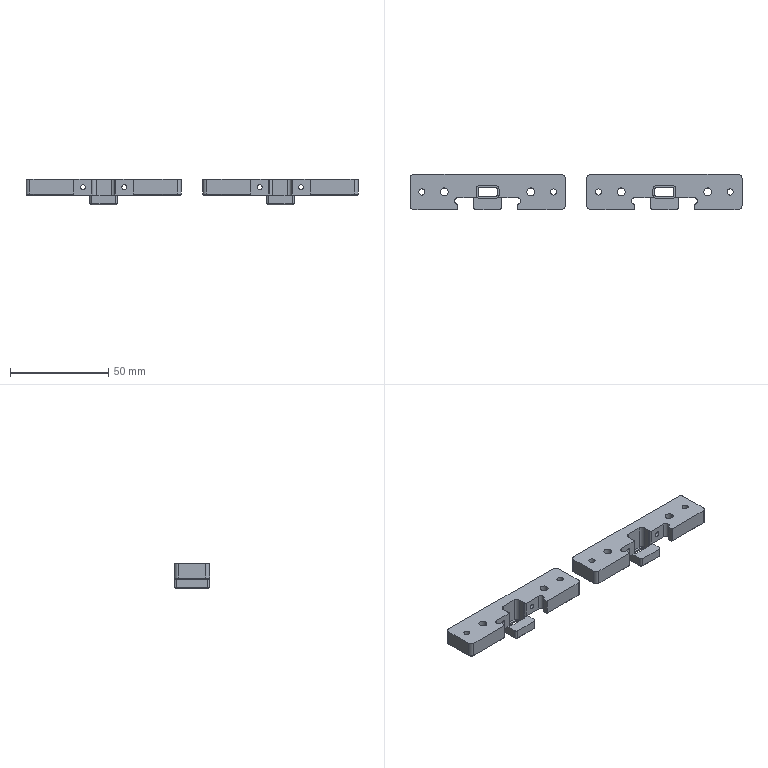NC program | NX | posted with a generic post | part box 169 x 18 x 12.9 mm
Whole program:
N10 G17 G21 G94 G90
(FLOOR_WALL_COPY , TOOL : D63)
N12 T01 M6
N14 G54
N16 G17 G0 G90 X-121. Y0. S6500 M3
N18 G43 Z30. H1
N20 Z4.
N22 G94 G1 Z1. F1250.
N24 X-118.
N26 X118.
N28 X121.
N30 Z4.
N32 G0 Z30.
N34 X-121.
N36 Z3.
N38 G1 Z0.
N40 X-118.
N42 X118.
N44 X121.
N46 Z3.
N48 G0 Z30.
N50 M5
(CAVITY_MILL_COPY_COPY_COPY_1 , TOOL : D6)
N52 T06 M6
N54 G54
N56 G17 G0 G90 X-2.829 Y15.196 S9500 M3
N58 G43 Z30. H6
N60 Z-0.6
N62 G94 G1 X-0.866 Y11.796 F1000.
N64 G3 X0. Y11.296 R1.
N66 G1 X35.32 F2000.
N68 G2 X39. Y12.94 R4.94
N70 G1 X51.
N72 G2 X54.68 Y11.296 R4.94
N74 G1 X86.504
N76 G2 X86.796 Y11.004 R0.292
N78 G1 Y-11.004
N80 G2 X86.504 Y-11.296 R0.292
N82 G1 X55.94
N84 Y-7.096
N86 Y7.096
N88 X82.596
N90 Y-7.096
N92 X55.94
N94 X60.14 Y-2.896
N96 Y2.896
N98 X78.396
N100 Y-2.896
N102 X60.14
N104 X62.84 Y-0.196
N106 Y0.196
N108 X75.696
N110 Y-0.196
N112 X62.84
N114 X55.94 Y-7.096
N116 Y-11.296
N118 X54.68
N120 G2 X51. Y-12.94 R4.94
N122 G1 X39.
N124 G2 X35.32 Y-11.296 R4.94
N126 G1 X-35.32
N128 G2 X-39. Y-12.94 R4.94
N130 G1 X-51.
N132 G2 X-54.68 Y-11.296 R4.94
N134 G1 X-86.504
N136 G2 X-86.796 Y-11.004 R0.292
N138 G1 Y11.004
N140 G2 X-86.504 Y11.296 R0.292
N142 G1 X-55.94
N144 Y7.096
N146 Y-7.096
N148 X-82.596
N150 Y7.096
N152 X-55.94
N154 X-60.14 Y2.896
N156 Y-2.896
N158 X-78.396
N160 Y2.896
N162 X-60.14
N164 X-62.84 Y0.196
N166 Y-0.196
N168 X-75.696
N170 Y0.196
N172 X-62.84
N174 X-55.94 Y7.096
N176 Y11.296
N178 X-54.68
N180 G2 X-51. Y12.94 R4.94
N182 G1 X-39.
N184 G2 X-35.32 Y11.296 R4.94
N186 G1 X0.
N188 Y7.096
N190 X34.06
N192 Y-7.096
N194 X34.9
N196 Y8.
N198 G2 X39. Y12.1 R4.1
N200 G1 X51.
N202 G2 X55.1 Y8. R4.1
N204 G1 Y-8.
N206 G2 X51. Y-12.1 R4.1
N208 G1 X39.
N210 G2 X34.9 Y-8. R4.1
N212 G1 Y-7.096
N214 X34.06
N216 X-34.06
N218 Y7.096
N220 X-34.9
N222 Y-8.
N224 G2 X-39. Y-12.1 R4.1
N226 G1 X-51.
N228 G2 X-55.1 Y-8. R4.1
N230 G1 Y8.
N232 G2 X-51. Y12.1 R4.1
N234 G1 X-39.
N236 G2 X-34.9 Y8. R4.1
N238 G1 Y7.096
N240 X-34.06
N242 X0.
N244 Y2.896
N246 X29.86
N248 Y-2.896
N250 X-29.86
N252 Y2.896
N254 X0.
N256 Y0.196
N258 X27.16
N260 Y-0.196
N262 X-27.16
N264 Y0.196
N266 X0.
N268 G3 X0.866 Y0.696 R1.
N270 G0 Z30.
N272 X-2.829 Y15.196
N274 Z-1.2
N276 G1 X-0.866 Y11.796 F1000.
N278 G3 X0. Y11.296 R1.
N280 G1 X35.32 F2000.
N282 G2 X39. Y12.94 R4.94
N284 G1 X51.
N286 G2 X54.68 Y11.296 R4.94
N288 G1 X86.504
N290 G2 X86.796 Y11.003 R0.292
N292 G1 Y-11.003
N294 G2 X86.504 Y-11.296 R0.292
N296 G1 X55.94
N298 Y-7.096
N300 Y7.096
N302 X82.596
N304 Y-7.096
N306 X55.94
N308 X60.14 Y-2.896
N310 Y2.896
N312 X78.396
N314 Y-2.896
N316 X60.14
N318 X62.84 Y-0.196
N320 Y0.196
N322 X75.696
N324 Y-0.196
N326 X62.84
N328 X55.94 Y-7.096
N330 Y-11.296
N332 X54.68
N334 G2 X51. Y-12.94 R4.94
N336 G1 X39.
N338 G2 X35.32 Y-11.296 R4.94
N340 G1 X-35.32
N342 G2 X-39. Y-12.94 R4.94
N344 G1 X-51.
N346 G2 X-54.68 Y-11.296 R4.94
N348 G1 X-86.504
N350 G2 X-86.796 Y-11.003 R0.292
N352 G1 Y11.003
N354 G2 X-86.504 Y11.296 R0.292
N356 G1 X-55.94
N358 Y7.096
N360 Y-7.096
N362 X-82.596
N364 Y7.096
N366 X-55.94
N368 X-60.14 Y2.896
N370 Y-2.896
N372 X-78.396
N374 Y2.896
N376 X-60.14
N378 X-62.84 Y0.196
N380 Y-0.196
N382 X-75.696
N384 Y0.196
N386 X-62.84
N388 X-55.94 Y7.096
N390 Y11.296
N392 X-54.68
N394 G2 X-51. Y12.94 R4.94
N396 G1 X-39.
N398 G2 X-35.32 Y11.296 R4.94
N400 G1 X0.
N402 Y7.096
N404 X34.06
N406 Y-7.096
N408 X34.9
N410 Y8.
N412 G2 X39. Y12.1 R4.1
N414 G1 X51.
N416 G2 X55.1 Y8. R4.1
N418 G1 Y-8.
N420 G2 X51. Y-12.1 R4.1
N422 G1 X39.
N424 G2 X34.9 Y-8. R4.1
N426 G1 Y-7.096
N428 X34.06
N430 X-34.06
N432 Y7.096
N434 X-34.9
N436 Y-8.
N438 G2 X-39. Y-12.1 R4.1
N440 G1 X-51.
N442 G2 X-55.1 Y-8. R4.1
N444 G1 Y8.
N446 G2 X-51. Y12.1 R4.1
N448 G1 X-39.
N450 G2 X-34.9 Y8. R4.1
N452 G1 Y7.096
N454 X-34.06
N456 X0.
N458 Y2.896
N460 X29.86
N462 Y-2.896
N464 X-29.86
N466 Y2.896
N468 X0.
N470 Y0.196
N472 X27.16
N474 Y-0.196
N476 X-27.16
N478 Y0.196
N480 X0.
N482 G3 X0.866 Y0.696 R1.
N484 G0 Z30.
N486 X-2.829 Y15.196
N488 Z-1.8
N490 G1 X-0.866 Y11.796 F1000.
N492 G3 X0. Y11.296 R1.
N494 G1 X35.32 F2000.
N496 G2 X39. Y12.94 R4.94
N498 G1 X51.
N500 G2 X54.68 Y11.296 R4.94
N502 G1 X86.504
N504 G2 X86.796 Y11.003 R0.293
N506 G1 Y-11.003
N508 G2 X86.504 Y-11.296 R0.293
N510 G1 X55.94
N512 Y-7.096
N514 Y7.096
N516 X82.596
N518 Y-7.096
N520 X55.94
N522 X60.14 Y-2.896
N524 Y2.896
N526 X78.396
N528 Y-2.896
N530 X60.14
N532 X62.84 Y-0.196
N534 Y0.196
N536 X75.696
N538 Y-0.196
N540 X62.84
N542 X55.94 Y-7.096
N544 Y-11.296
N546 X54.68
N548 G2 X51. Y-12.94 R4.94
N550 G1 X39.
N552 G2 X35.32 Y-11.296 R4.94
N554 G1 X-35.32
N556 G2 X-39. Y-12.94 R4.94
N558 G1 X-51.
N560 G2 X-54.68 Y-11.296 R4.94
N562 G1 X-86.504
N564 G2 X-86.796 Y-11.003 R0.293
N566 G1 Y11.003
N568 G2 X-86.504 Y11.296 R0.293
N570 G1 X-55.94
N572 Y7.096
N574 Y-7.096
N576 X-82.596
N578 Y7.096
N580 X-55.94
N582 X-60.14 Y2.896
N584 Y-2.896
N586 X-78.396
N588 Y2.896
N590 X-60.14
N592 X-62.84 Y0.196
N594 Y-0.196
N596 X-75.696
N598 Y0.196
N600 X-62.84
N602 X-55.94 Y7.096
N604 Y11.296
N606 X-54.68
N608 G2 X-51. Y12.94 R4.94
N610 G1 X-39.
N612 G2 X-35.32 Y11.296 R4.94
N614 G1 X0.
N616 Y7.096
N618 X34.06
N620 Y-7.096
N622 X34.9
N624 Y8.
N626 G2 X39. Y12.1 R4.1
N628 G1 X51.
N630 G2 X55.1 Y8. R4.1
N632 G1 Y-8.
N634 G2 X51. Y-12.1 R4.1
N636 G1 X39.
N638 G2 X34.9 Y-8. R4.1
N640 G1 Y-7.096
N642 X34.06
N644 X-34.06
N646 Y7.096
N648 X-34.9
N650 Y-8.
N652 G2 X-39. Y-12.1 R4.1
N654 G1 X-51.
N656 G2 X-55.1 Y-8. R4.1
N658 G1 Y8.
N660 G2 X-51. Y12.1 R4.1
N662 G1 X-39.
N664 G2 X-34.9 Y8. R4.1
N666 G1 Y7.096
N668 X-34.06
N670 X0.
N672 Y2.896
N674 X29.86
N676 Y-2.896
N678 X-29.86
N680 Y2.896
N682 X0.
N684 Y0.196
N686 X27.16
N688 Y-0.196
N690 X-27.16
N692 Y0.196
N694 X0.
N696 G3 X0.866 Y0.696 R1.
N698 G0 Z30.
N700 X-2.829 Y15.196
N702 Z-2.4
N704 G1 X-0.866 Y11.796 F1000.
N706 G3 X0. Y11.296 R1.
N708 G1 X35.321 F2000.
N710 G2 X39. Y12.94 R4.94
N712 G1 X51.
N714 G2 X54.679 Y11.296 R4.94
N716 G1 X86.503
N718 G2 X86.797 Y11.003 R0.293
N720 G1 Y-11.003
N722 G2 X86.503 Y-11.296 R0.293
N724 G1 X55.94
N726 Y-7.096
N728 Y7.096
N730 X82.597
N732 Y-7.096
N734 X55.94
N736 X60.14 Y-2.896
N738 Y2.896
N740 X78.397
N742 Y-2.896
N744 X60.14
N746 X62.84 Y-0.196
N748 Y0.196
N750 X75.697
N752 Y-0.196
N754 X62.84
N756 X60.14 Y-2.896
N758 X55.94 Y-7.096
N760 Y-11.296
N762 X54.679
N764 G2 X51. Y-12.94 R4.94
N766 G1 X39.
N768 G2 X35.321 Y-11.296 R4.94
N770 G1 X-35.321
N772 G2 X-39. Y-12.94 R4.94
N774 G1 X-51.
N776 G2 X-54.679 Y-11.296 R4.94
N778 G1 X-86.504
N780 G2 X-86.797 Y-11.003 R0.293
N782 G1 Y11.003
N784 G2 X-86.504 Y11.296 R0.293
N786 G1 X-55.94
N788 Y7.096
N790 Y-7.096
N792 X-82.597
N794 Y7.096
N796 X-55.94
N798 X-60.14 Y2.896
N800 Y-2.896
N802 X-78.397
N804 Y2.896
N806 X-60.14
N808 X-62.84 Y0.196
N810 Y-0.196
N812 X-75.697
N814 Y0.196
N816 X-62.84
N818 X-55.94 Y7.096
N820 Y11.296
N822 X-54.679
N824 G2 X-51. Y12.94 R4.94
N826 G1 X-39.
N828 G2 X-35.321 Y11.296 R4.94
N830 G1 X0.
N832 Y7.096
N834 X34.06
N836 Y-7.096
N838 X34.9
N840 Y8.
N842 G2 X39. Y12.1 R4.1
N844 G1 X51.
N846 G2 X55.1 Y8. R4.1
N848 G1 Y-8.
N850 G2 X51. Y-12.1 R4.1
N852 G1 X39.
N854 G2 X34.9 Y-8. R4.1
N856 G1 Y-7.096
N858 X34.06
N860 X-34.06
N862 Y7.096
N864 X-34.9
N866 Y-8.
N868 G2 X-39. Y-12.1 R4.1
N870 G1 X-51.
N872 G2 X-55.1 Y-8. R4.1
N874 G1 Y8.
N876 G2 X-51. Y12.1 R4.1
N878 G1 X-39.
N880 G2 X-34.9 Y8. R4.1
N882 G1 Y7.096
N884 X-34.06
N886 X0.
N888 Y2.896
N890 X29.86
N892 Y-2.896
N894 X-29.86
N896 Y2.896
N898 X0.
N900 Y0.196
N902 X27.16
N904 Y-0.196
N906 X-27.16
N908 Y0.196
N910 X0.
N912 G3 X0.866 Y0.696 R1.
N914 G0 Z30.
N916 X-2.829 Y15.196
N918 Z-3.
N920 G1 X-0.866 Y11.796 F1000.
N922 G3 X0. Y11.296 R1.
N924 G1 X35.321 F2000.
N926 G2 X39. Y12.94 R4.94
N928 G1 X51.
N930 G2 X54.679 Y11.296 R4.94
N932 G1 X86.503
N934 G2 X86.797 Y11.003 R0.293
N936 G1 Y-11.003
N938 G2 X86.503 Y-11.296 R0.293
N940 G1 X55.94
N942 Y-7.096
N944 Y7.096
N946 X82.597
N948 Y-7.096
N950 X55.94
N952 X60.14 Y-2.896
N954 Y2.896
N956 X78.397
N958 Y-2.896
N960 X60.14
N962 X62.84 Y-0.196
N964 Y0.196
N966 X75.697
N968 Y-0.196
N970 X62.84
N972 X55.94 Y-7.096
N974 Y-11.296
N976 X54.679
N978 G2 X51. Y-12.94 R4.94
N980 G1 X39.
N982 G2 X35.321 Y-11.296 R4.94
N984 G1 X-35.321
N986 G2 X-39. Y-12.94 R4.94
N988 G1 X-51.
N990 G2 X-54.679 Y-11.296 R4.94
N992 G1 X-86.503
N994 G2 X-86.797 Y-11.003 R0.293
N996 G1 Y11.003
N998 G2 X-86.503 Y11.296 R0.293
N1000 G1 X-55.94
N1002 Y7.096
N1004 Y-7.096
N1006 X-82.597
N1008 Y7.096
N1010 X-55.94
N1012 X-60.14 Y2.896
N1014 Y-2.896
N1016 X-78.397
N1018 Y2.896
N1020 X-60.14
N1022 X-62.84 Y0.196
N1024 Y-0.196
N1026 X-75.697
N1028 Y0.196
N1030 X-62.84
N1032 X-55.94 Y7.096
N1034 Y11.296
N1036 X-54.679
N1038 G2 X-51. Y12.94 R4.94
N1040 G1 X-39.
N1042 G2 X-35.321 Y11.296 R4.94
N1044 G1 X0.
N1046 Y7.096
N1048 X34.06
N1050 Y-7.096
N1052 X34.9
N1054 Y8.
N1056 G2 X39. Y12.1 R4.1
N1058 G1 X51.
N1060 G2 X55.1 Y8. R4.1
N1062 G1 Y-8.
N1064 G2 X51. Y-12.1 R4.1
N1066 G1 X39.
N1068 G2 X34.9 Y-8. R4.1
N1070 G1 Y-7.096
N1072 X34.06
N1074 X-34.06
N1076 Y7.096
N1078 X-34.9
N1080 Y-8.
N1082 G2 X-39. Y-12.1 R4.1
N1084 G1 X-51.
N1086 G2 X-55.1 Y-8. R4.1
N1088 G1 Y8.
N1090 G2 X-51. Y12.1 R4.1
N1092 G1 X-39.
N1094 G2 X-34.9 Y8. R4.1
N1096 G1 Y7.096
N1098 X-34.06
N1100 X0.
N1102 Y2.896
N1104 X29.86
N1106 Y-2.896
N1108 X-29.86
N1110 Y2.896
N1112 X0.
N1114 Y0.196
N1116 X27.16
N1118 Y-0.196
N1120 X-27.16
N1122 Y0.196
N1124 X0.
N1126 G3 X0.866 Y0.696 R1.
N1128 G0 Z30.
N1130 X-2.829 Y15.197
N1132 Z-3.6
N1134 G1 X-0.866 Y11.797 F1000.
N1136 G3 X0. Y11.297 R1.
N1138 G1 X35.321 F2000.
N1140 G2 X39. Y12.94 R4.94
N1142 G1 X51.
N1144 G2 X54.679 Y11.297 R4.94
N1146 G1 X86.503
N1148 G2 X86.797 Y11.003 R0.294
N1150 G1 Y-11.003
N1152 G2 X86.503 Y-11.297 R0.294
N1154 G1 X55.94
N1156 Y-7.097
N1158 Y7.097
N1160 X82.597
N1162 Y-7.097
N1164 X55.94
N1166 X60.14 Y-2.897
N1168 Y2.897
N1170 X78.397
N1172 Y-2.897
N1174 X60.14
N1176 X62.84 Y-0.197
N1178 Y0.197
N1180 X75.697
N1182 Y-0.197
N1184 X62.84
N1186 X55.94 Y-7.097
N1188 Y-11.297
N1190 X54.679
N1192 G2 X51. Y-12.94 R4.94
N1194 G1 X39.
N1196 G2 X35.321 Y-11.297 R4.94
N1198 G1 X-35.321
N1200 G2 X-39. Y-12.94 R4.94
N1202 G1 X-51.
N1204 G2 X-54.679 Y-11.297 R4.94
N1206 G1 X-86.503
N1208 G2 X-86.797 Y-11.003 R0.294
N1210 G1 Y11.003
N1212 G2 X-86.503 Y11.297 R0.294
N1214 G1 X-55.94
N1216 Y7.097
N1218 Y-7.097
N1220 X-82.597
N1222 Y7.097
N1224 X-55.94
N1226 X-60.14 Y2.897
N1228 Y-2.897
N1230 X-78.397
N1232 Y2.897
N1234 X-60.14
N1236 X-62.84 Y0.197
N1238 Y-0.197
N1240 X-75.697
N1242 Y0.197
N1244 X-62.84
N1246 X-55.94 Y7.097
N1248 Y11.297
N1250 X-54.679
N1252 G2 X-51. Y12.94 R4.94
N1254 G1 X-39.
N1256 G2 X-35.321 Y11.297 R4.94
N1258 G1 X0.
N1260 Y7.097
N1262 X34.06
N1264 Y-7.097
N1266 X34.9
N1268 Y8.
N1270 G2 X39. Y12.1 R4.1
N1272 G1 X51.
N1274 G2 X55.1 Y8. R4.1
N1276 G1 Y-8.
N1278 G2 X51. Y-12.1 R4.1
N1280 G1 X39.
N1282 G2 X34.9 Y-8. R4.1
N1284 G1 Y-7.097
N1286 X34.06
N1288 X-34.06
N1290 Y7.097
N1292 X-34.9
N1294 Y-8.
N1296 G2 X-39. Y-12.1 R4.1
N1298 G1 X-51.
N1300 G2 X-55.1 Y-8. R4.1
N1302 G1 Y8.
N1304 G2 X-51. Y12.1 R4.1
N1306 G1 X-39.
N1308 G2 X-34.9 Y8. R4.1
N1310 G1 Y7.097
N1312 X-34.06
N1314 X0.
N1316 Y2.897
N1318 X29.86
N1320 Y-2.897
N1322 X-29.86
N1324 Y2.897
N1326 X0.
N1328 Y0.197
N1330 X27.16
N1332 Y-0.197
N1334 X-27.16
N1336 Y0.197
N1338 X0.
N1340 G3 X0.866 Y0.697 R1.
N1342 G0 Z30.
N1344 X-2.829 Y15.197
N1346 Z-4.2
N1348 G1 X-0.866 Y11.797 F1000.
N1350 G3 X0. Y11.297 R1.
N1352 G1 X35.321 F2000.
N1354 G2 X39. Y12.94 R4.94
N1356 G1 X51.
N1358 G2 X54.679 Y11.297 R4.94
N1360 G1 X86.503
N1362 G2 X86.797 Y11.003 R0.294
N1364 G1 Y-11.003
N1366 G2 X86.503 Y-11.297 R0.294
N1368 G1 X55.94
N1370 Y-7.097
N1372 Y7.097
N1374 X82.597
N1376 Y-7.097
N1378 X55.94
N1380 X60.14 Y-2.897
N1382 Y2.897
N1384 X78.397
N1386 Y-2.897
N1388 X60.14
N1390 X62.84 Y-0.197
N1392 Y0.197
N1394 X75.697
N1396 Y-0.197
N1398 X62.84
N1400 X55.94 Y-7.097
N1402 Y-11.297
N1404 X54.679
N1406 G2 X51. Y-12.94 R4.94
N1408 G1 X39.
N1410 G2 X35.321 Y-11.297 R4.94
N1412 G1 X-35.321
N1414 G2 X-39. Y-12.94 R4.94
N1416 G1 X-51.
N1418 G2 X-54.679 Y-11.297 R4.94
N1420 G1 X-86.503
N1422 G2 X-86.797 Y-11.003 R0.294
N1424 G1 Y11.003
N1426 G2 X-86.503 Y11.297 R0.294
N1428 G1 X-55.94
N1430 Y7.097
N1432 Y-7.097
N1434 X-82.597
N1436 Y7.097
N1438 X-55.94
N1440 X-60.14 Y2.897
N1442 Y-2.897
N1444 X-78.397
N1446 Y2.897
N1448 X-60.14
N1450 X-62.84 Y0.197
N1452 Y-0.197
N1454 X-75.697
N1456 Y0.197
N1458 X-62.84
N1460 X-55.94 Y7.097
N1462 Y11.297
N1464 X-54.679
N1466 G2 X-51. Y12.94 R4.94
N1468 G1 X-39.
N1470 G2 X-35.321 Y11.297 R4.94
N1472 G1 X0.
N1474 Y7.097
N1476 X34.06
N1478 Y-7.097
N1480 X34.9
N1482 Y8.
N1484 G2 X39. Y12.1 R4.1
N1486 G1 X51.
N1488 G2 X55.1 Y8. R4.1
N1490 G1 Y-8.
N1492 G2 X51. Y-12.1 R4.1
N1494 G1 X39.
N1496 G2 X34.9 Y-8. R4.1
N1498 G1 Y-7.097
N1500 X34.06
N1502 X-34.06
N1504 Y7.097
N1506 X-34.9
N1508 Y-8.
N1510 G2 X-39. Y-12.1 R4.1
N1512 G1 X-51.
N1514 G2 X-55.1 Y-8. R4.1
N1516 G1 Y8.
N1518 G2 X-51. Y12.1 R4.1
N1520 G1 X-39.
N1522 G2 X-34.9 Y8. R4.1
N1524 G1 Y7.097
N1526 X-34.06
N1528 X0.
N1530 Y2.897
N1532 X29.86
N1534 Y-2.897
N1536 X-29.86
N1538 Y2.897
N1540 X0.
N1542 Y0.197
N1544 X27.16
N1546 Y-0.197
N1548 X-27.16
N1550 Y0.197
N1552 X0.
N1554 G3 X0.866 Y0.697 R1.
N1556 G0 Z30.
N1558 X-2.829 Y15.197
N1560 Z-4.8
N1562 G1 X-0.866 Y11.797 F1000.
N1564 G3 X0. Y11.297 R1.
N1566 G1 X35.321 F2000.
N1568 G2 X39. Y12.94 R4.94
N1570 G1 X51.
N1572 G2 X54.679 Y11.297 R4.94
N1574 G1 X86.503
N1576 G2 X86.797 Y11.003 R0.294
N1578 G1 Y-11.003
N1580 G2 X86.503 Y-11.297 R0.294
N1582 G1 X55.94
N1584 Y-7.097
N1586 Y7.097
N1588 X82.597
N1590 Y-7.097
N1592 X55.94
N1594 X60.14 Y-2.897
N1596 Y2.897
N1598 X78.397
N1600 Y-2.897
N1602 X60.14
N1604 X62.84 Y-0.197
N1606 Y0.197
N1608 X75.697
N1610 Y-0.197
N1612 X62.84
N1614 X55.94 Y-7.097
N1616 Y-11.297
N1618 X54.679
N1620 G2 X51. Y-12.94 R4.94
N1622 G1 X39.
N1624 G2 X35.321 Y-11.297 R4.94
N1626 G1 X-35.321
N1628 G2 X-39. Y-12.94 R4.94
N1630 G1 X-51.
N1632 G2 X-54.679 Y-11.297 R4.94
N1634 G1 X-86.503
N1636 G2 X-86.797 Y-11.003 R0.294
N1638 G1 Y11.003
N1640 G2 X-86.503 Y11.297 R0.294
N1642 G1 X-55.94
N1644 Y7.097
N1646 Y-7.097
N1648 X-82.597
N1650 Y7.097
N1652 X-55.94
N1654 X-60.14 Y2.897
N1656 Y-2.897
N1658 X-78.397
N1660 Y2.897
N1662 X-60.14
N1664 X-62.84 Y0.197
N1666 Y-0.197
N1668 X-75.697
N1670 Y0.197
N1672 X-62.84
N1674 X-55.94 Y7.097
N1676 Y11.297
N1678 X-54.679
N1680 G2 X-51. Y12.94 R4.94
N1682 G1 X-39.
N1684 G2 X-35.321 Y11.297 R4.94
N1686 G1 X0.
N1688 Y7.097
N1690 X34.06
N1692 Y-7.097
N1694 X34.9
N1696 Y8.
N1698 G2 X39. Y12.1 R4.1
N1700 G1 X51.
N1702 G2 X55.1 Y8. R4.1
N1704 G1 Y-8.
N1706 G2 X51. Y-12.1 R4.1
N1708 G1 X39.
N1710 G2 X34.9 Y-8. R4.1
N1712 G1 Y-7.097
N1714 X34.06
N1716 X-34.06
N1718 Y7.097
N1720 X-34.9
N1722 Y-8.
N1724 G2 X-39. Y-12.1 R4.1
N1726 G1 X-51.
N1728 G2 X-55.1 Y-8. R4.1
N1730 G1 Y8.
N1732 G2 X-51. Y12.1 R4.1
N1734 G1 X-39.
N1736 G2 X-34.9 Y8. R4.1
N1738 G1 Y7.097
N1740 X-34.06
N1742 X0.
N1744 Y2.897
N1746 X29.86
N1748 Y-2.897
N1750 X-29.86
N1752 Y2.897
N1754 X0.
N1756 Y0.197
N1758 X27.16
N1760 Y-0.197
N1762 X-27.16
N1764 Y0.197
N1766 X0.
N1768 G3 X0.866 Y0.697 R1.
N1770 G0 Z30.
(ZLEVEL_PROFILE_COPY_COPY_COPY_COPY_COPY_COPY , TOOL : D6)
N1772 X34.448 Y-8.665
N1774 Z-3.4
N1776 G1 Z-4.9 F1000.
N1778 X34.7 Y-8.52
N1780 G3 X35. Y-8. R0.6
N1782 G1 Y8. F1200.
N1784 G2 X39. Y12. R4.
N1786 G1 X51.
N1788 G2 X55. Y8. R4.
N1790 G1 Y-8.
N1792 G2 X51. Y-12. R4.
N1794 G1 X39.
N1796 G2 X35. Y-8. R4.
N1798 G3 X34.7 Y-7.48 R0.6
N1800 G1 X34.4 Y-7.307
N1802 Z-3.4
N1804 G0 Z30.
N1806 X-34.448 Y8.665
N1808 Z-3.4
N1810 G1 Z-4.9 F1000.
N1812 X-34.7 Y8.52
N1814 G3 X-35. Y8. R0.6
N1816 G1 Y-8. F1200.
N1818 G2 X-39. Y-12. R4.
N1820 G1 X-51.
N1822 G2 X-55. Y-8. R4.
N1824 G1 Y8.
N1826 G2 X-51. Y12. R4.
N1828 G1 X-39.
N1830 G2 X-35. Y8. R4.
N1832 G3 X-34.7 Y7.48 R0.6
N1834 G1 X-34.4 Y7.307
N1836 Z-3.4
N1838 G0 Z30.
(FLOOR_WALL_1 , TOOL : D6)
N1840 X-85.267 Y-12.324
N1842 Z-3.4
N1844 G1 Z-4.9 F1000.
N1846 X-84.297 Y-11.763
N1848 G3 X-83.997 Y-11.244 R0.6
N1850 G1 Y11.244
N1852 G2 X-82.5 Y11.5 R4.5
N1854 G1 X-81.124
N1856 Y-11.5
N1858 X-78.252
N1860 Y11.5
N1862 X-75.379
N1864 Y-11.5
N1866 X-72.507
N1868 Y11.5
N1870 X-69.634
N1872 Y-11.5
N1874 X-66.761
N1876 Y11.5
N1878 X-63.889
N1880 Y-11.5
N1882 X-61.016
N1884 Y11.5
N1886 X-58.143
N1888 Y-11.5
N1890 X-57.2
N1892 Y-6.
N1894 X-55.3
N1896 Y8.
N1898 G2 X-55.271 Y8.5 R4.3
N1900 G1 Y11.5
N1902 G3 X-55.571 Y12.02 R0.6
N1904 G1 X-57.269 Y13.
N1906 Z-3.4
N1908 G0 Z30.
N1910 X-58.7 Y-8.483
N1912 Z-3.4
N1914 G1 Z-4.9
N1916 X-55.3 Y-6.52
N1918 G3 X-55. Y-6. R0.6
N1920 G1 Y8.
N1922 G2 X-52.99 Y11.47 R4.
N1924 G3 X-52.688 Y11.989 R0.6
N1926 G1 X-52.685 Y13.236
N1928 Z-3.4
N1930 G0 Z30.
N1932 X-4.733 Y12.324
N1934 Z-3.4
N1936 G1 Z-4.9
N1938 X-5.703 Y11.763
N1940 G3 X-6.003 Y11.244 R0.6
N1942 G1 Y-11.244
N1944 G2 X-7.499 Y-11.5 R4.5
N1946 G1 X-8.876
N1948 Y11.5
N1950 X-11.748
N1952 Y-11.5
N1954 X-14.621
N1956 Y11.5
N1958 X-17.493
N1960 Y-11.5
N1962 X-20.366
N1964 Y11.5
N1966 X-23.239
N1968 Y-11.5
N1970 X-26.111
N1972 Y11.5
N1974 X-28.984
N1976 Y-11.5
N1978 X-31.857
N1980 Y11.5
N1982 X-34.729
N1984 Y8.5
N1986 G3 X-34.429 Y7.98 R0.6
N1988 G1 Z-3.4
N1990 G0 Z30.
N1992 X-37.315 Y13.236
N1994 Z-3.4
N1996 G1 Z-4.9
N1998 X-37.312 Y11.989
N2000 G3 X-37.01 Y11.47 R0.6
N2002 G2 X-35. Y8. R4.
N2004 G1 Y-6.
N2006 G3 X-34.7 Y-6.52 R0.6
N2008 G1 X-31.3 Y-8.483
N2010 Z-3.4
N2012 G0 Z30.
N2014 X4.733 Y-12.324
N2016 Z-3.4
N2018 G1 Z-4.9
N2020 X5.703 Y-11.763
N2022 G3 X6.003 Y-11.244 R0.6
N2024 G1 Y11.244
N2026 G2 X7.5 Y11.5 R4.5
N2028 G1 X8.876
N2030 Y-11.5
N2032 X11.748
N2034 Y11.5
N2036 X14.621
N2038 Y-11.5
N2040 X17.493
N2042 Y11.5
N2044 X20.366
N2046 Y-11.5
N2048 X23.239
N2050 Y11.5
N2052 X26.111
N2054 Y-11.5
N2056 X28.984
N2058 Y11.5
N2060 X31.857
N2062 Y-11.5
N2064 X32.8
N2066 Y-6.
N2068 X34.7
N2070 Y8.
N2072 G2 X34.729 Y8.5 R4.3
N2074 G1 Y11.5
N2076 G3 X34.429 Y12.02 R0.6
N2078 G1 X32.731 Y13.
N2080 Z-3.4
N2082 G0 Z30.
N2084 X31.3 Y-8.483
N2086 Z-3.4
N2088 G1 Z-4.9
N2090 X34.7 Y-6.52
N2092 G3 X35. Y-6. R0.6
N2094 G1 Y8.
N2096 G2 X37.01 Y11.47 R4.
N2098 G3 X37.312 Y11.989 R0.6
N2100 G1 X37.315 Y13.236
N2102 Z-3.4
N2104 G0 Z30.
N2106 X85.267 Y12.324
N2108 Z-3.4
N2110 G1 Z-4.9
N2112 X84.297 Y11.763
N2114 G3 X83.997 Y11.244 R0.6
N2116 G1 Y-11.244
N2118 G2 X82.501 Y-11.5 R4.5
N2120 G1 X81.124
N2122 Y11.5
N2124 X78.252
N2126 Y-11.5
N2128 X75.379
N2130 Y11.5
N2132 X72.507
N2134 Y-11.5
N2136 X69.634
N2138 Y11.5
N2140 X66.761
N2142 Y-11.5
N2144 X63.889
N2146 Y11.5
N2148 X61.016
N2150 Y-11.5
N2152 X58.143
N2154 Y11.5
N2156 X55.271
N2158 Y8.5
N2160 G3 X55.571 Y7.98 R0.6
N2162 G1 Z-3.4
N2164 G0 Z30.
N2166 X52.685 Y13.236
N2168 Z-3.4
N2170 G1 Z-4.9
N2172 X52.688 Y11.989
N2174 G3 X52.99 Y11.47 R0.6
N2176 G2 X55. Y8. R4.
N2178 G1 Y-6.
N2180 G3 X55.3 Y-6.52 R0.6
N2182 G1 X58.7 Y-8.483
N2184 Z-3.4
N2186 G0 Z30.
N2188 M5
(HOLE_MILLING , TOOL : D4)
N2190 T04 M6
N2192 G54
N2194 G17 G0 G90 X-78.5 Y0. S9500 M3
N2196 G43 Z30. H4
N2198 Z-4.4
N2200 G94 G3 X-79. Y0.5 R0.5 F1500.
N2202 X-79.5 Y0. R0.5
N2204 X-79.5 Y0. Z-4.8 I1. J0.
N2206 X-79.5 Y0. Z-5.2 I1. J0.
N2208 X-79.5 Y0. Z-5.6 I1. J0.
N2210 X-79.5 Y0. Z-6. I1. J0.
N2212 X-79.5 Y0. Z-6.4 I1. J0.
N2214 X-79.5 Y0. Z-6.8 I1. J0.
N2216 X-79.5 Y0. Z-7.2 I1. J0.
N2218 X-79.5 Y0. Z-7.6 I1. J0.
N2220 X-79.5 Y0. Z-8. I1. J0.
N2222 X-79.5 Y0. Z-8.4 I1. J0.
N2224 X-79.5 Y0. Z-8.8 I1. J0.
N2226 X-78.5 Y-1. Z-8.9 R1.
N2228 X-77.5 Y0. R1.
N2230 X-78.5 Y-1. R-1.
N2232 X-78. Y-0.5 R0.5
N2234 X-78.5 Y0. R0.5
N2236 G0 Z30.
N2238 X-11.5
N2240 Z-4.4
N2242 G3 X-12. Y0.5 R0.5
N2244 X-12.5 Y0. R0.5
N2246 X-12.5 Y0. Z-4.8 I1. J0.
N2248 X-12.5 Y0. Z-5.2 I1. J0.
N2250 X-12.5 Y0. Z-5.6 I1. J0.
N2252 X-12.5 Y0. Z-6. I1. J0.
N2254 X-12.5 Y0. Z-6.4 I1. J0.
N2256 X-12.5 Y0. Z-6.8 I1. J0.
N2258 X-12.5 Y0. Z-7.2 I1. J0.
N2260 X-12.5 Y0. Z-7.6 I1. J0.
N2262 X-12.5 Y0. Z-8. I1. J0.
N2264 X-12.5 Y0. Z-8.4 I1. J0.
N2266 X-12.5 Y0. Z-8.8 I1. J0.
N2268 X-11.5 Y-1. Z-8.9 R1.
N2270 X-10.5 Y0. R1.
N2272 X-11.5 Y-1. R-1.
N2274 X-11. Y-0.5 R0.5
N2276 X-11.5 Y0. R0.5
N2278 G0 Z30.
N2280 X11.5
N2282 Z-4.4
N2284 G3 X11. Y0.5 R0.5
N2286 X10.5 Y0. R0.5
N2288 X10.5 Y0. Z-4.8 I1. J0.
N2290 X10.5 Y0. Z-5.2 I1. J0.
N2292 X10.5 Y0. Z-5.6 I1. J0.
N2294 X10.5 Y0. Z-6. I1. J0.
N2296 X10.5 Y0. Z-6.4 I1. J0.
N2298 X10.5 Y0. Z-6.8 I1. J0.
N2300 X10.5 Y0. Z-7.2 I1. J0.
N2302 X10.5 Y0. Z-7.6 I1. J0.
N2304 X10.5 Y0. Z-8. I1. J0.
N2306 X10.5 Y0. Z-8.4 I1. J0.
N2308 X10.5 Y0. Z-8.8 I1. J0.
N2310 X11.5 Y-1. Z-8.9 R1.
N2312 X12.5 Y0. R1.
N2314 X11.5 Y-1. R-1.
N2316 X12. Y-0.5 R0.5
N2318 X11.5 Y0. R0.5
N2320 G0 Z30.
N2322 X78.5
N2324 Z-4.4
N2326 G3 X78. Y0.5 R0.5
N2328 X77.5 Y0. R0.5
N2330 X77.5 Y0. Z-4.8 I1. J0.
N2332 X77.5 Y0. Z-5.2 I1. J0.
N2334 X77.5 Y0. Z-5.6 I1. J0.
N2336 X77.5 Y0. Z-6. I1. J0.
N2338 X77.5 Y0. Z-6.4 I1. J0.
N2340 X77.5 Y0. Z-6.8 I1. J0.
N2342 X77.5 Y0. Z-7.2 I1. J0.
N2344 X77.5 Y0. Z-7.6 I1. J0.
N2346 X77.5 Y0. Z-8. I1. J0.
N2348 X77.5 Y0. Z-8.4 I1. J0.
N2350 X77.5 Y0. Z-8.8 I1. J0.
N2352 X78.5 Y-1. Z-8.9 R1.
N2354 X79.5 Y0. R1.
N2356 X78.5 Y-1. R-1.
N2358 X79. Y-0.5 R0.5
N2360 X78.5 Y0. R0.5
N2362 G0 Z30.
N2364 M5
(ZLEVEL_PROFILE_1_COPY_1_COPY_COPY_COPY , TOOL : D4A45)
N2366 T02 M6
N2368 G54
N2370 G17 G0 G90 X47.864 Y0.691 S9500 M3
N2372 G43 Z30. H2
N2374 Z0.
N2376 G94 G1 Z-1. F1000.
N2378 X48.65 Y1.145
N2380 G3 X48.85 Y1.491 R0.4
N2382 G1 X41.15
N2384 X41.124 Y1.495
N2386 X41.105 Y1.476
N2388 X41.109 Y1.45
N2390 Y-1.45
N2392 X41.105 Y-1.476
N2394 X41.124 Y-1.495
N2396 X41.15 Y-1.491
N2398 X48.85
N2400 X48.876 Y-1.495
N2402 X48.895 Y-1.476
N2404 X48.891 Y-1.45
N2406 Y1.45
N2408 X48.895 Y1.476
N2410 X48.876 Y1.495
N2412 X48.85 Y1.491
N2414 G3 X48.504 Y1.291 R0.4
N2416 G1 X48.091 Y0.578
N2418 Z0.
N2420 G0 Z30.
N2422 X-42.136 Y0.691
N2424 Z0.
N2426 G1 Z-1.
N2428 X-41.35 Y1.145
N2430 G3 X-41.15 Y1.491 R0.4
N2432 G1 X-48.85
N2434 X-48.876 Y1.495
N2436 X-48.895 Y1.476
N2438 X-48.891 Y1.45
N2440 Y-1.45
N2442 X-48.895 Y-1.476
N2444 X-48.876 Y-1.495
N2446 X-48.85 Y-1.491
N2448 X-41.15
N2450 X-41.124 Y-1.495
N2452 X-41.105 Y-1.476
N2454 X-41.109 Y-1.45
N2456 Y1.45
N2458 X-41.105 Y1.476
N2460 X-41.124 Y1.495
N2462 X-41.15 Y1.491
N2464 G3 X-41.496 Y1.291 R0.4
N2466 G1 X-41.909 Y0.578
N2468 Z0.
N2470 G0 Z30.
N2472 X-36.834 Y8.639
N2474 Z0.
N2476 G1 Z-1.
N2478 X-37.341 Y8.346
N2480 G3 X-37.541 Y8. R0.4
N2482 G1 Y-8.
N2484 G2 X-39. Y-9.459 R1.459
N2486 G1 X-51.
N2488 G2 X-52.459 Y-8. R1.459
N2490 G1 Y8.
N2492 G2 X-51. Y9.459 R1.459
N2494 G1 X-39.
N2496 G2 X-37.541 Y8. R1.459
N2498 G3 X-37.341 Y7.654 R0.4
N2500 G1 X-36.741 Y7.307
N2502 Z0.
N2504 G0 Z30.
N2506 X38.361 Y10.166
N2508 Z0.
N2510 G1 Z-1.
N2512 X38.654 Y9.659
N2514 G3 X39. Y9.459 R0.4
N2516 G1 X51.
N2518 G2 X52.459 Y8. R1.459
N2520 G1 Y-8.
N2522 G2 X51. Y-9.459 R1.459
N2524 G1 X39.
N2526 G2 X37.541 Y-8. R1.459
N2528 G1 Y8.
N2530 G2 X39. Y9.459 R1.459
N2532 G3 X39.346 Y9.659 R0.4
N2534 G1 X39.693 Y10.259
N2536 Z0.
N2538 G0 Z30.
(ZLEVEL_PROFILE_1_COPY_1_COPY_COPY_COPY_COPY , TOOL : D4A45)
N2540 X-67.106 Y-0.272
N2542 Z-4.9
N2544 G1 Z-5.9
N2546 X-67.346 Y-0.891
N2548 G3 X-67. Y-1.091 R0.4
N2550 X-65.909 Y0. R1.091
N2552 X-67. Y-1.091 R-1.091
N2554 X-66.654 Y-0.891 R0.4
N2556 G1 X-66.894 Y-0.272
N2558 Z-4.9
N2560 G0 Z30.
N2562 X-12.444 Y-0.806
N2564 Z-4.9
N2566 G1 Z-5.9
N2568 X-11.846 Y-1.841
N2570 G3 X-11.5 Y-2.041 R0.4
N2572 X-9.459 Y0. R2.041
N2574 X-11.5 Y-2.041 R-2.041
N2576 X-11.154 Y-1.841 R0.4
N2578 G1 X-10.556 Y-0.806
N2580 Z-4.9
N2582 G0 Z30.
N2584 X-79.306 Y0.944
N2586 Z-4.9
N2588 G1 Z-5.9
N2590 X-80.341 Y0.346
N2592 G3 X-80.541 Y0. R0.4
N2594 X-78.5 Y-2.041 R2.041
N2596 X-80.541 Y0. R-2.041
N2598 X-80.341 Y-0.346 R0.4
N2600 G1 X-79.306 Y-0.944
N2602 Z-4.9
N2604 G0 Z30.
N2606 X-23.106 Y-0.272
N2608 Z-4.9
N2610 G1 Z-5.9
N2612 X-23.346 Y-0.891
N2614 G3 X-23. Y-1.091 R0.4
N2616 X-21.909 Y0. R1.091
N2618 X-23. Y-1.091 R-1.091
N2620 X-22.654 Y-0.891 R0.4
N2622 G1 X-22.894 Y-0.272
N2624 Z-4.9
N2626 G0 Z30.
N2628 X79.306 Y-0.944
N2630 Z-4.9
N2632 G1 Z-5.9
N2634 X80.341 Y-0.346
N2636 G3 X80.541 Y0. R0.4
N2638 X78.5 Y2.041 R2.041
N2640 X80.541 Y0. R-2.041
N2642 X80.341 Y0.346 R0.4
N2644 G1 X79.306 Y0.944
N2646 Z-4.9
N2648 G0 Z30.
N2650 X12.444 Y0.806
N2652 Z-4.9
N2654 G1 Z-5.9
N2656 X11.846 Y1.841
N2658 G3 X11.5 Y2.041 R0.4
N2660 X9.459 Y0. R2.041
N2662 X11.5 Y2.041 R-2.041
N2664 X11.154 Y1.841 R0.4
N2666 G1 X10.556 Y0.806
N2668 Z-4.9
N2670 G0 Z30.
N2672 X23.106 Y0.272
N2674 Z-4.9
N2676 G1 Z-5.9
N2678 X23.346 Y0.891
N2680 G3 X23. Y1.091 R0.4
N2682 X21.909 Y0. R1.091
N2684 X23. Y1.091 R-1.091
N2686 X22.654 Y0.891 R0.4
N2688 G1 X22.894 Y0.272
N2690 Z-4.9
N2692 G0 Z30.
N2694 X67.106
N2696 Z-4.9
N2698 G1 Z-5.9
N2700 X67.346 Y0.891
N2702 G3 X67. Y1.091 R0.4
N2704 X65.909 Y0. R1.091
N2706 X67. Y1.091 R-1.091
N2708 X66.654 Y0.891 R0.4
N2710 G1 X66.894 Y0.272
N2712 Z-4.9
N2714 G0 Z30.
N2716 X53.931 Y10.259
N2718 Z-4.9
N2720 G1 Z-5.9
N2722 X53.682 Y9.559
N2724 G3 X53.855 Y9.459 R0.2
N2726 G1 X82.5
N2728 G2 X84.959 Y7. R2.459
N2730 G1 Y-7.
N2732 G2 X82.5 Y-9.459 R2.459
N2734 G1 X60.199
N2736 G2 X59.241 Y-8.501 R0.964
N2738 G1 Y-6.199
N2740 G2 X60.202 Y-5.241 R0.961
N2742 G3 X60.841 Y-4.598 R0.641
N2744 X60.2 Y-3.959 R0.641
N2746 G1 X54.208
N2748 X54.154 Y-3.956
N2750 X54.108 Y-3.985
N2752 X54.7 Y-4.759
N2754 Z-4.9
N2756 G0 Z30.
N2758 X35.3
N2760 Z-4.9
N2762 G1 Z-5.9
N2764 X35.891 Y-3.985
N2766 X35.845 Y-3.956
N2768 X35.791 Y-3.959
N2770 X29.8
N2772 G3 X29.159 Y-4.6 R0.641
N2774 X29.801 Y-5.241 R0.641
N2776 G2 X30.759 Y-6.199 R0.957
N2778 G1 Y-8.501
N2780 G2 X29.801 Y-9.459 R0.958
N2782 G1 X7.5
N2784 G2 X5.041 Y-7. R2.459
N2786 G1 Y7.
N2788 G2 X7.5 Y9.459 R2.459
N2790 G1 X36.146
N2792 G3 X36.319 Y9.559 R0.2
N2794 G1 X36.069 Y10.259
N2796 Z-4.9
N2798 G0 Z30.
N2800 X-36.069
N2802 Z-4.9
N2804 G1 Z-5.9
N2806 X-36.319 Y9.559
N2808 G3 X-36.146 Y9.459 R0.2
N2810 G1 X-7.5
N2812 G2 X-5.041 Y7. R2.459
N2814 G1 Y-7.
N2816 G2 X-7.5 Y-9.459 R2.459
N2818 G1 X-29.801
N2820 G2 X-30.759 Y-8.501 R0.958
N2822 G1 Y-6.199
N2824 G2 X-29.797 Y-5.241 R0.961
N2826 G3 X-29.159 Y-4.597 R0.641
N2828 X-29.8 Y-3.959 R0.641
N2830 G1 X-35.791
N2832 X-35.845 Y-3.956
N2834 X-35.891 Y-3.985
N2836 X-35.3 Y-4.759
N2838 Z-4.9
N2840 G0 Z30.
N2842 X-54.7
N2844 Z-4.9
N2846 G1 Z-5.9
N2848 X-54.108 Y-3.985
N2850 X-54.154 Y-3.956
N2852 X-54.208 Y-3.959
N2854 X-60.2
N2856 G3 X-60.841 Y-4.6 R0.641
N2858 X-60.199 Y-5.241 R0.641
N2860 G2 X-59.241 Y-6.199 R0.957
N2862 G1 Y-8.501
N2864 G2 X-60.199 Y-9.459 R0.964
N2866 G1 X-82.5
N2868 G2 X-84.959 Y-7. R2.459
N2870 G1 Y7.
N2872 G2 X-82.5 Y9.459 R2.459
N2874 G1 X-53.855
N2876 G3 X-53.682 Y9.559 R0.2
N2878 G1 X-53.931 Y10.259
N2880 Z-4.9
N2882 G0 Z30.
N2884 M5
N2886 M2